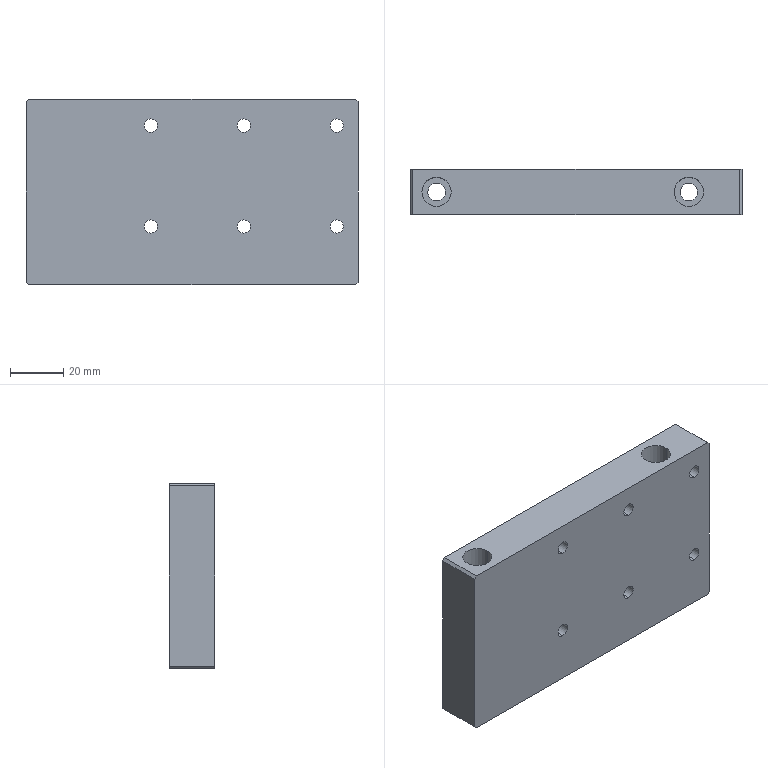Part | STEP file | 1 solid | 32 faces | box 125 x 17 x 70 mm | volume 135841 mm3 | cylinder 20 | plane 12 | commonest cylinder face diameters 5 x12 6.6 x4 11 x4